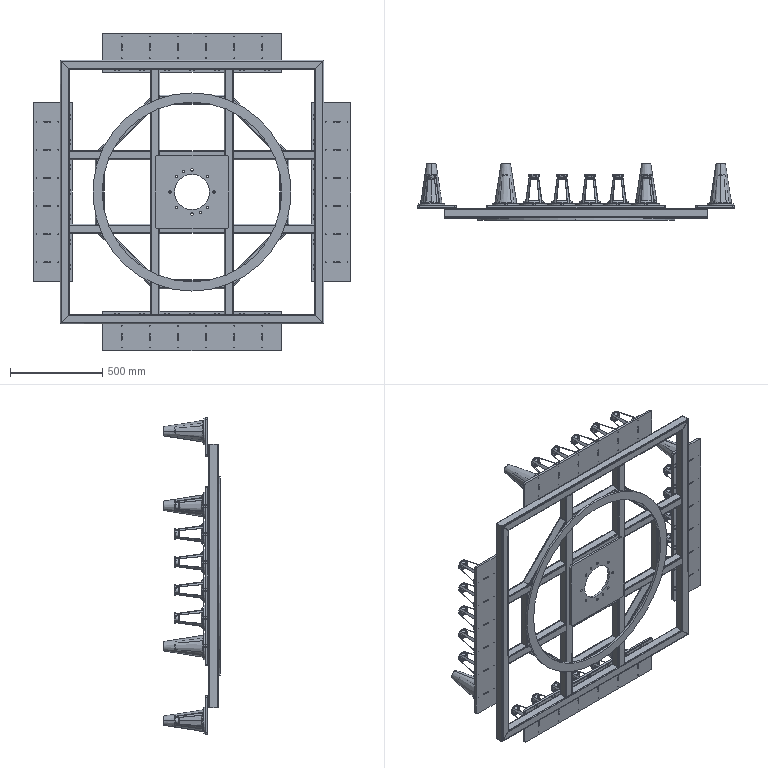Part | SolidWorks | 154 solids | 3774 faces | volume 27946605 mm3 | plane 1668 | cylinder 1650 | cone 384 | torus 72 | commonest cylinder face diameters 4.2 x368 4 x288 10 x208 5.5 x128 5 x112 3.3 x96